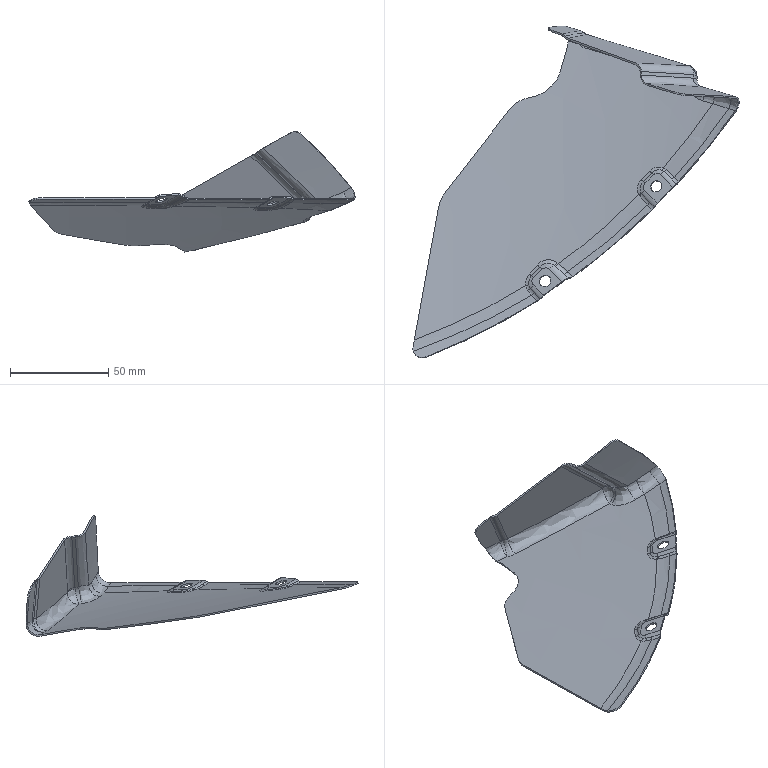Part | STEP file | FNA5401153 | 1 solid | 184 faces | box 165.89 x 168.782 x 61.393 mm | volume 13779 mm3 | spline 170 | cylinder 8 | plane 6 | commonest cylinder face diameters 6 x4 8 x2 9.6 x2